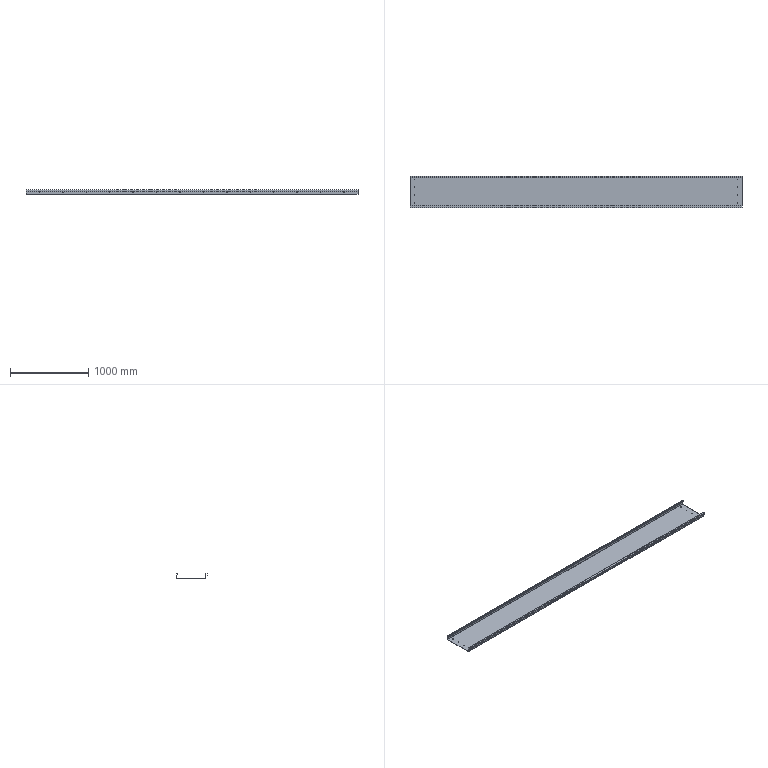Part | STEP file | TS-S47 | 1 solid | 126 faces | box 4250 x 403 x 62 mm | volume 4791334 mm3 | cylinder 84 | plane 42 | commonest cylinder face diameters 5.4 x56 7 x16 0.4 x6 4.4 x6